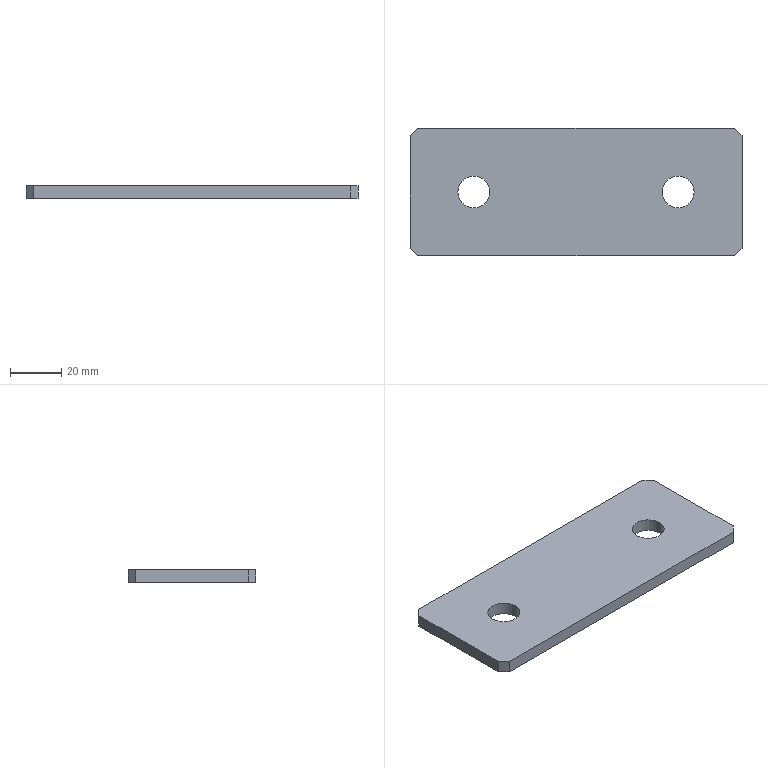Part | SolidWorks | features Extrusion 1 | 1 solid | 14 faces | box 130 x 50 x 5 mm | volume 31183 mm3 | plane 10 | cylinder 4 | commonest cylinder face diameters 12.5 x4
STEP:
#1=CARTESIAN_POINT('',(33.75,0.,-2.5));
#2=VERTEX_POINT('',#1);
#3=CARTESIAN_POINT('',(46.25,0.,-2.5));
#4=VERTEX_POINT('',#3);
#5=CARTESIAN_POINT('',(40.,0.,-2.5));
#6=DIRECTION('',(0.,0.,1.));
#7=DIRECTION('',(-1.,0.,0.));
#8=AXIS2_PLACEMENT_3D('',#5,#6,#7);
#9=CIRCLE('',#8,6.25);
#10=EDGE_CURVE('',#2,#4,#9,.T.);
#11=ORIENTED_EDGE('',*,*,#10,.F.);
#12=CARTESIAN_POINT('',(33.75,0.,2.5));
#13=VERTEX_POINT('',#12);
#14=CARTESIAN_POINT('',(33.75,0.,-2.5));
#15=DIRECTION('',(0.,0.,1.));
#16=VECTOR('',#15,1000.);
#17=LINE('',#14,#16);
#18=EDGE_CURVE('',#2,#13,#17,.T.);
#19=ORIENTED_EDGE('',*,*,#18,.T.);
#20=CARTESIAN_POINT('',(46.25,0.,2.5));
#21=VERTEX_POINT('',#20);
#22=CARTESIAN_POINT('',(40.,0.,2.5));
#23=DIRECTION('',(0.,0.,1.));
#24=DIRECTION('',(-1.,0.,0.));
#25=AXIS2_PLACEMENT_3D('',#22,#23,#24);
#26=CIRCLE('',#25,6.25);
#27=EDGE_CURVE('',#13,#21,#26,.T.);
#28=ORIENTED_EDGE('',*,*,#27,.T.);
#29=CARTESIAN_POINT('',(46.25,0.,-2.5));
#30=DIRECTION('',(0.,0.,1.));
#31=VECTOR('',#30,1000.);
#32=LINE('',#29,#31);
#33=EDGE_CURVE('',#4,#21,#32,.T.);
#34=ORIENTED_EDGE('',*,*,#33,.F.);
#35=EDGE_LOOP('',(#11,#19,#28,#34));
#36=FACE_OUTER_BOUND('',#35,.T.);
#37=CARTESIAN_POINT('',(40.,0.,-2.5));
#38=DIRECTION('',(0.,0.,1.));
#39=DIRECTION('',(1.,0.,0.));
#40=AXIS2_PLACEMENT_3D('',#37,#38,#39);
#41=CYLINDRICAL_SURFACE('',#40,6.25);
#42=ADVANCED_FACE('',(#36),#41,.F.);
#43=CARTESIAN_POINT('',(-46.25,0.,-2.5));
#44=VERTEX_POINT('',#43);
#45=CARTESIAN_POINT('',(-33.75,0.,-2.5));
#46=VERTEX_POINT('',#45);
#47=CARTESIAN_POINT('',(-40.,0.,-2.5));
#48=DIRECTION('',(0.,0.,1.));
#49=DIRECTION('',(-1.,0.,0.));
#50=AXIS2_PLACEMENT_3D('',#47,#48,#49);
#51=CIRCLE('',#50,6.25);
#52=EDGE_CURVE('',#44,#46,#51,.T.);
#53=ORIENTED_EDGE('',*,*,#52,.F.);
#54=CARTESIAN_POINT('',(-46.25,0.,2.5));
#55=VERTEX_POINT('',#54);
#56=CARTESIAN_POINT('',(-46.25,0.,-2.5));
#57=DIRECTION('',(0.,0.,1.));
#58=VECTOR('',#57,1000.);
#59=LINE('',#56,#58);
#60=EDGE_CURVE('',#44,#55,#59,.T.);
#61=ORIENTED_EDGE('',*,*,#60,.T.);
#62=CARTESIAN_POINT('',(-33.75,0.,2.5));
#63=VERTEX_POINT('',#62);
#64=CARTESIAN_POINT('',(-40.,0.,2.5));
#65=DIRECTION('',(0.,0.,1.));
#66=DIRECTION('',(-1.,0.,0.));
#67=AXIS2_PLACEMENT_3D('',#64,#65,#66);
#68=CIRCLE('',#67,6.25);
#69=EDGE_CURVE('',#55,#63,#68,.T.);
#70=ORIENTED_EDGE('',*,*,#69,.T.);
#71=CARTESIAN_POINT('',(-33.75,0.,-2.5));
#72=DIRECTION('',(0.,0.,1.));
#73=VECTOR('',#72,1000.);
#74=LINE('',#71,#73);
#75=EDGE_CURVE('',#46,#63,#74,.T.);
#76=ORIENTED_EDGE('',*,*,#75,.F.);
#77=EDGE_LOOP('',(#53,#61,#70,#76));
#78=FACE_OUTER_BOUND('',#77,.T.);
#79=CARTESIAN_POINT('',(-40.,0.,-2.5));
#80=DIRECTION('',(0.,0.,1.));
#81=DIRECTION('',(1.,0.,0.));
#82=AXIS2_PLACEMENT_3D('',#79,#80,#81);
#83=CYLINDRICAL_SURFACE('',#82,6.25);
#84=ADVANCED_FACE('',(#78),#83,.F.);
#85=CARTESIAN_POINT('',(-65.,-22.,2.5));
#86=VERTEX_POINT('',#85);
#87=CARTESIAN_POINT('',(-62.,-25.,2.5));
#88=VERTEX_POINT('',#87);
#89=CARTESIAN_POINT('',(-65.,-22.,2.5));
#90=DIRECTION('',(0.7071,-0.7071,0.));
#91=VECTOR('',#90,1000.);
#92=LINE('',#89,#91);
#93=EDGE_CURVE('',#86,#88,#92,.T.);
#94=ORIENTED_EDGE('',*,*,#93,.F.);
#95=CARTESIAN_POINT('',(-65.,-22.,-2.5));
#96=VERTEX_POINT('',#95);
#97=CARTESIAN_POINT('',(-65.,-22.,-2.5));
#98=DIRECTION('',(0.,0.,1.));
#99=VECTOR('',#98,1000.);
#100=LINE('',#97,#99);
#101=EDGE_CURVE('',#96,#86,#100,.T.);
#102=ORIENTED_EDGE('',*,*,#101,.F.);
#103=CARTESIAN_POINT('',(-62.,-25.,-2.5));
#104=VERTEX_POINT('',#103);
#105=CARTESIAN_POINT('',(-65.,-22.,-2.5));
#106=DIRECTION('',(0.7071,-0.7071,0.));
#107=VECTOR('',#106,1000.);
#108=LINE('',#105,#107);
#109=EDGE_CURVE('',#96,#104,#108,.T.);
#110=ORIENTED_EDGE('',*,*,#109,.T.);
#111=CARTESIAN_POINT('',(-62.,-25.,-2.5));
#112=DIRECTION('',(0.,0.,1.));
#113=VECTOR('',#112,1000.);
#114=LINE('',#111,#113);
#115=EDGE_CURVE('',#104,#88,#114,.T.);
#116=ORIENTED_EDGE('',*,*,#115,.T.);
#117=EDGE_LOOP('',(#94,#102,#110,#116));
#118=FACE_OUTER_BOUND('',#117,.T.);
#119=CARTESIAN_POINT('',(-65.,-22.,-2.5));
#120=DIRECTION('',(-0.7071,-0.7071,0.));
#121=DIRECTION('',(0.7071,-0.7071,0.));
#122=AXIS2_PLACEMENT_3D('',#119,#120,#121);
#123=PLANE('',#122);
#124=ADVANCED_FACE('',(#118),#123,.T.);
#125=CARTESIAN_POINT('',(-65.,22.,2.5));
#126=VERTEX_POINT('',#125);
#127=CARTESIAN_POINT('',(-65.,22.,2.5));
#128=DIRECTION('',(0.,-1.,0.));
#129=VECTOR('',#128,1000.);
#130=LINE('',#127,#129);
#131=EDGE_CURVE('',#126,#86,#130,.T.);
#132=ORIENTED_EDGE('',*,*,#131,.F.);
#133=CARTESIAN_POINT('',(-65.,22.,-2.5));
#134=VERTEX_POINT('',#133);
#135=CARTESIAN_POINT('',(-65.,22.,-2.5));
#136=DIRECTION('',(0.,0.,1.));
#137=VECTOR('',#136,1000.);
#138=LINE('',#135,#137);
#139=EDGE_CURVE('',#134,#126,#138,.T.);
#140=ORIENTED_EDGE('',*,*,#139,.F.);
#141=CARTESIAN_POINT('',(-65.,22.,-2.5));
#142=DIRECTION('',(0.,-1.,0.));
#143=VECTOR('',#142,1000.);
#144=LINE('',#141,#143);
#145=EDGE_CURVE('',#134,#96,#144,.T.);
#146=ORIENTED_EDGE('',*,*,#145,.T.);
#147=ORIENTED_EDGE('',*,*,#101,.T.);
#148=EDGE_LOOP('',(#132,#140,#146,#147));
#149=FACE_OUTER_BOUND('',#148,.T.);
#150=CARTESIAN_POINT('',(-65.,22.,-2.5));
#151=DIRECTION('',(-1.,0.,0.));
#152=DIRECTION('',(0.,0.,1.));
#153=AXIS2_PLACEMENT_3D('',#150,#151,#152);
#154=PLANE('',#153);
#155=ADVANCED_FACE('',(#149),#154,.T.);
#156=CARTESIAN_POINT('',(-62.,25.,2.5));
#157=VERTEX_POINT('',#156);
#158=CARTESIAN_POINT('',(-62.,25.,2.5));
#159=DIRECTION('',(-0.7071,-0.7071,0.));
#160=VECTOR('',#159,1000.);
#161=LINE('',#158,#160);
#162=EDGE_CURVE('',#157,#126,#161,.T.);
#163=ORIENTED_EDGE('',*,*,#162,.F.);
#164=CARTESIAN_POINT('',(-62.,25.,-2.5));
#165=VERTEX_POINT('',#164);
#166=CARTESIAN_POINT('',(-62.,25.,-2.5));
#167=DIRECTION('',(0.,0.,1.));
#168=VECTOR('',#167,1000.);
#169=LINE('',#166,#168);
#170=EDGE_CURVE('',#165,#157,#169,.T.);
#171=ORIENTED_EDGE('',*,*,#170,.F.);
#172=CARTESIAN_POINT('',(-62.,25.,-2.5));
#173=DIRECTION('',(-0.7071,-0.7071,0.));
#174=VECTOR('',#173,1000.);
#175=LINE('',#172,#174);
#176=EDGE_CURVE('',#165,#134,#175,.T.);
#177=ORIENTED_EDGE('',*,*,#176,.T.);
#178=ORIENTED_EDGE('',*,*,#139,.T.);
#179=EDGE_LOOP('',(#163,#171,#177,#178));
#180=FACE_OUTER_BOUND('',#179,.T.);
#181=CARTESIAN_POINT('',(-62.,25.,-2.5));
#182=DIRECTION('',(-0.7071,0.7071,0.));
#183=DIRECTION('',(-0.7071,-0.7071,0.));
#184=AXIS2_PLACEMENT_3D('',#181,#182,#183);
#185=PLANE('',#184);
#186=ADVANCED_FACE('',(#180),#185,.T.);
#187=CARTESIAN_POINT('',(62.,25.,2.5));
#188=VERTEX_POINT('',#187);
#189=CARTESIAN_POINT('',(62.,25.,2.5));
#190=DIRECTION('',(-1.,0.,0.));
#191=VECTOR('',#190,1000.);
#192=LINE('',#189,#191);
#193=EDGE_CURVE('',#188,#157,#192,.T.);
#194=ORIENTED_EDGE('',*,*,#193,.F.);
#195=CARTESIAN_POINT('',(62.,25.,-2.5));
#196=VERTEX_POINT('',#195);
#197=CARTESIAN_POINT('',(62.,25.,-2.5));
#198=DIRECTION('',(0.,0.,1.));
#199=VECTOR('',#198,1000.);
#200=LINE('',#197,#199);
#201=EDGE_CURVE('',#196,#188,#200,.T.);
#202=ORIENTED_EDGE('',*,*,#201,.F.);
#203=CARTESIAN_POINT('',(62.,25.,-2.5));
#204=DIRECTION('',(-1.,0.,0.));
#205=VECTOR('',#204,1000.);
#206=LINE('',#203,#205);
#207=EDGE_CURVE('',#196,#165,#206,.T.);
#208=ORIENTED_EDGE('',*,*,#207,.T.);
#209=ORIENTED_EDGE('',*,*,#170,.T.);
#210=EDGE_LOOP('',(#194,#202,#208,#209));
#211=FACE_OUTER_BOUND('',#210,.T.);
#212=CARTESIAN_POINT('',(62.,25.,-2.5));
#213=DIRECTION('',(0.,1.,0.));
#214=DIRECTION('',(0.,0.,1.));
#215=AXIS2_PLACEMENT_3D('',#212,#213,#214);
#216=PLANE('',#215);
#217=ADVANCED_FACE('',(#211),#216,.T.);
#218=CARTESIAN_POINT('',(65.,22.,2.5));
#219=VERTEX_POINT('',#218);
#220=CARTESIAN_POINT('',(65.,22.,2.5));
#221=DIRECTION('',(-0.7071,0.7071,0.));
#222=VECTOR('',#221,1000.);
#223=LINE('',#220,#222);
#224=EDGE_CURVE('',#219,#188,#223,.T.);
#225=ORIENTED_EDGE('',*,*,#224,.F.);
#226=CARTESIAN_POINT('',(65.,22.,-2.5));
#227=VERTEX_POINT('',#226);
#228=CARTESIAN_POINT('',(65.,22.,-2.5));
#229=DIRECTION('',(0.,0.,1.));
#230=VECTOR('',#229,1000.);
#231=LINE('',#228,#230);
#232=EDGE_CURVE('',#227,#219,#231,.T.);
#233=ORIENTED_EDGE('',*,*,#232,.F.);
#234=CARTESIAN_POINT('',(65.,22.,-2.5));
#235=DIRECTION('',(-0.7071,0.7071,0.));
#236=VECTOR('',#235,1000.);
#237=LINE('',#234,#236);
#238=EDGE_CURVE('',#227,#196,#237,.T.);
#239=ORIENTED_EDGE('',*,*,#238,.T.);
#240=ORIENTED_EDGE('',*,*,#201,.T.);
#241=EDGE_LOOP('',(#225,#233,#239,#240));
#242=FACE_OUTER_BOUND('',#241,.T.);
#243=CARTESIAN_POINT('',(65.,22.,-2.5));
#244=DIRECTION('',(0.7071,0.7071,0.));
#245=DIRECTION('',(-0.7071,0.7071,0.));
#246=AXIS2_PLACEMENT_3D('',#243,#244,#245);
#247=PLANE('',#246);
#248=ADVANCED_FACE('',(#242),#247,.T.);
#249=CARTESIAN_POINT('',(65.,-22.,2.5));
#250=VERTEX_POINT('',#249);
#251=CARTESIAN_POINT('',(65.,-22.,2.5));
#252=DIRECTION('',(0.,1.,0.));
#253=VECTOR('',#252,1000.);
#254=LINE('',#251,#253);
#255=EDGE_CURVE('',#250,#219,#254,.T.);
#256=ORIENTED_EDGE('',*,*,#255,.F.);
#257=CARTESIAN_POINT('',(65.,-22.,-2.5));
#258=VERTEX_POINT('',#257);
#259=CARTESIAN_POINT('',(65.,-22.,-2.5));
#260=DIRECTION('',(0.,0.,1.));
#261=VECTOR('',#260,1000.);
#262=LINE('',#259,#261);
#263=EDGE_CURVE('',#258,#250,#262,.T.);
#264=ORIENTED_EDGE('',*,*,#263,.F.);
#265=CARTESIAN_POINT('',(65.,-22.,-2.5));
#266=DIRECTION('',(0.,1.,0.));
#267=VECTOR('',#266,1000.);
#268=LINE('',#265,#267);
#269=EDGE_CURVE('',#258,#227,#268,.T.);
#270=ORIENTED_EDGE('',*,*,#269,.T.);
#271=ORIENTED_EDGE('',*,*,#232,.T.);
#272=EDGE_LOOP('',(#256,#264,#270,#271));
#273=FACE_OUTER_BOUND('',#272,.T.);
#274=CARTESIAN_POINT('',(65.,-22.,-2.5));
#275=DIRECTION('',(1.,0.,0.));
#276=DIRECTION('',(0.,0.,-1.));
#277=AXIS2_PLACEMENT_3D('',#274,#275,#276);
#278=PLANE('',#277);
#279=ADVANCED_FACE('',(#273),#278,.T.);
#280=CARTESIAN_POINT('',(62.,-25.,2.5));
#281=VERTEX_POINT('',#280);
#282=CARTESIAN_POINT('',(62.,-25.,2.5));
#283=DIRECTION('',(0.7071,0.7071,0.));
#284=VECTOR('',#283,1000.);
#285=LINE('',#282,#284);
#286=EDGE_CURVE('',#281,#250,#285,.T.);
#287=ORIENTED_EDGE('',*,*,#286,.F.);
#288=CARTESIAN_POINT('',(62.,-25.,-2.5));
#289=VERTEX_POINT('',#288);
#290=CARTESIAN_POINT('',(62.,-25.,-2.5));
#291=DIRECTION('',(0.,0.,1.));
#292=VECTOR('',#291,1000.);
#293=LINE('',#290,#292);
#294=EDGE_CURVE('',#289,#281,#293,.T.);
#295=ORIENTED_EDGE('',*,*,#294,.F.);
#296=CARTESIAN_POINT('',(62.,-25.,-2.5));
#297=DIRECTION('',(0.7071,0.7071,0.));
#298=VECTOR('',#297,1000.);
#299=LINE('',#296,#298);
#300=EDGE_CURVE('',#289,#258,#299,.T.);
#301=ORIENTED_EDGE('',*,*,#300,.T.);
#302=ORIENTED_EDGE('',*,*,#263,.T.);
#303=EDGE_LOOP('',(#287,#295,#301,#302));
#304=FACE_OUTER_BOUND('',#303,.T.);
#305=CARTESIAN_POINT('',(62.,-25.,-2.5));
#306=DIRECTION('',(0.7071,-0.7071,0.));
#307=DIRECTION('',(0.7071,0.7071,0.));
#308=AXIS2_PLACEMENT_3D('',#305,#306,#307);
#309=PLANE('',#308);
#310=ADVANCED_FACE('',(#304),#309,.T.);
#311=CARTESIAN_POINT('',(-62.,-25.,2.5));
#312=DIRECTION('',(1.,0.,0.));
#313=VECTOR('',#312,1000.);
#314=LINE('',#311,#313);
#315=EDGE_CURVE('',#88,#281,#314,.T.);
#316=ORIENTED_EDGE('',*,*,#315,.F.);
#317=ORIENTED_EDGE('',*,*,#115,.F.);
#318=CARTESIAN_POINT('',(-62.,-25.,-2.5));
#319=DIRECTION('',(1.,0.,0.));
#320=VECTOR('',#319,1000.);
#321=LINE('',#318,#320);
#322=EDGE_CURVE('',#104,#289,#321,.T.);
#323=ORIENTED_EDGE('',*,*,#322,.T.);
#324=ORIENTED_EDGE('',*,*,#294,.T.);
#325=EDGE_LOOP('',(#316,#317,#323,#324));
#326=FACE_OUTER_BOUND('',#325,.T.);
#327=CARTESIAN_POINT('',(-62.,-25.,-2.5));
#328=DIRECTION('',(0.,-1.,0.));
#329=DIRECTION('',(0.,0.,-1.));
#330=AXIS2_PLACEMENT_3D('',#327,#328,#329);
#331=PLANE('',#330);
#332=ADVANCED_FACE('',(#326),#331,.T.);
#333=CARTESIAN_POINT('',(40.,0.,-2.5));
#334=DIRECTION('',(0.,0.,1.));
#335=DIRECTION('',(-1.,0.,0.));
#336=AXIS2_PLACEMENT_3D('',#333,#334,#335);
#337=CIRCLE('',#336,6.25);
#338=EDGE_CURVE('',#4,#2,#337,.T.);
#339=ORIENTED_EDGE('',*,*,#338,.T.);
#340=ORIENTED_EDGE('',*,*,#10,.T.);
#341=EDGE_LOOP('',(#339,#340));
#342=FACE_BOUND('',#341,.T.);
#343=CARTESIAN_POINT('',(-40.,0.,-2.5));
#344=DIRECTION('',(0.,0.,1.));
#345=DIRECTION('',(-1.,0.,0.));
#346=AXIS2_PLACEMENT_3D('',#343,#344,#345);
#347=CIRCLE('',#346,6.25);
#348=EDGE_CURVE('',#46,#44,#347,.T.);
#349=ORIENTED_EDGE('',*,*,#348,.T.);
#350=ORIENTED_EDGE('',*,*,#52,.T.);
#351=EDGE_LOOP('',(#349,#350));
#352=FACE_BOUND('',#351,.T.);
#353=ORIENTED_EDGE('',*,*,#109,.F.);
#354=ORIENTED_EDGE('',*,*,#145,.F.);
#355=ORIENTED_EDGE('',*,*,#176,.F.);
#356=ORIENTED_EDGE('',*,*,#207,.F.);
#357=ORIENTED_EDGE('',*,*,#238,.F.);
#358=ORIENTED_EDGE('',*,*,#269,.F.);
#359=ORIENTED_EDGE('',*,*,#300,.F.);
#360=ORIENTED_EDGE('',*,*,#322,.F.);
#361=EDGE_LOOP('',(#353,#354,#355,#356,#357,#358,#359,#360));
#362=FACE_OUTER_BOUND('',#361,.T.);
#363=CARTESIAN_POINT('',(0.,0.,-2.5));
#364=DIRECTION('',(0.,0.,1.));
#365=DIRECTION('',(1.,0.,0.));
#366=AXIS2_PLACEMENT_3D('',#363,#364,#365);
#367=PLANE('',#366);
#368=ADVANCED_FACE('',(#342,#352,#362),#367,.F.);
#369=CARTESIAN_POINT('',(40.,0.,2.5));
#370=DIRECTION('',(0.,0.,1.));
#371=DIRECTION('',(-1.,0.,0.));
#372=AXIS2_PLACEMENT_3D('',#369,#370,#371);
#373=CIRCLE('',#372,6.25);
#374=EDGE_CURVE('',#21,#13,#373,.T.);
#375=ORIENTED_EDGE('',*,*,#374,.F.);
#376=ORIENTED_EDGE('',*,*,#27,.F.);
#377=EDGE_LOOP('',(#375,#376));
#378=FACE_BOUND('',#377,.T.);
#379=CARTESIAN_POINT('',(-40.,0.,2.5));
#380=DIRECTION('',(0.,0.,1.));
#381=DIRECTION('',(-1.,0.,0.));
#382=AXIS2_PLACEMENT_3D('',#379,#380,#381);
#383=CIRCLE('',#382,6.25);
#384=EDGE_CURVE('',#63,#55,#383,.T.);
#385=ORIENTED_EDGE('',*,*,#384,.F.);
#386=ORIENTED_EDGE('',*,*,#69,.F.);
#387=EDGE_LOOP('',(#385,#386));
#388=FACE_BOUND('',#387,.T.);
#389=ORIENTED_EDGE('',*,*,#93,.T.);
#390=ORIENTED_EDGE('',*,*,#315,.T.);
#391=ORIENTED_EDGE('',*,*,#286,.T.);
#392=ORIENTED_EDGE('',*,*,#255,.T.);
#393=ORIENTED_EDGE('',*,*,#224,.T.);
#394=ORIENTED_EDGE('',*,*,#193,.T.);
#395=ORIENTED_EDGE('',*,*,#162,.T.);
#396=ORIENTED_EDGE('',*,*,#131,.T.);
#397=EDGE_LOOP('',(#389,#390,#391,#392,#393,#394,#395,#396));
#398=FACE_OUTER_BOUND('',#397,.T.);
#399=CARTESIAN_POINT('',(0.,0.,2.5));
#400=DIRECTION('',(0.,0.,1.));
#401=DIRECTION('',(1.,0.,0.));
#402=AXIS2_PLACEMENT_3D('',#399,#400,#401);
#403=PLANE('',#402);
#404=ADVANCED_FACE('',(#378,#388,#398),#403,.T.);
#405=ORIENTED_EDGE('',*,*,#60,.F.);
#406=ORIENTED_EDGE('',*,*,#348,.F.);
#407=ORIENTED_EDGE('',*,*,#75,.T.);
#408=ORIENTED_EDGE('',*,*,#384,.T.);
#409=EDGE_LOOP('',(#405,#406,#407,#408));
#410=FACE_OUTER_BOUND('',#409,.T.);
#411=CARTESIAN_POINT('',(-40.,0.,-2.5));
#412=DIRECTION('',(0.,0.,1.));
#413=DIRECTION('',(1.,0.,0.));
#414=AXIS2_PLACEMENT_3D('',#411,#412,#413);
#415=CYLINDRICAL_SURFACE('',#414,6.25);
#416=ADVANCED_FACE('',(#410),#415,.F.);
#417=ORIENTED_EDGE('',*,*,#18,.F.);
#418=ORIENTED_EDGE('',*,*,#338,.F.);
#419=ORIENTED_EDGE('',*,*,#33,.T.);
#420=ORIENTED_EDGE('',*,*,#374,.T.);
#421=EDGE_LOOP('',(#417,#418,#419,#420));
#422=FACE_OUTER_BOUND('',#421,.T.);
#423=CARTESIAN_POINT('',(40.,0.,-2.5));
#424=DIRECTION('',(0.,0.,1.));
#425=DIRECTION('',(1.,0.,0.));
#426=AXIS2_PLACEMENT_3D('',#423,#424,#425);
#427=CYLINDRICAL_SURFACE('',#426,6.25);
#428=ADVANCED_FACE('',(#422),#427,.F.);
#429=CLOSED_SHELL('',(#42,#84,#124,#155,#186,#217,#248,#279,#310,#332,#368,#404,#416,#428));
#430=MANIFOLD_SOLID_BREP('',#429);
#431=CARTESIAN_POINT('',(0.,0.,0.));
#432=DIRECTION('',(0.,0.,1.));
#433=DIRECTION('',(1.,0.,0.));
#434=AXIS2_PLACEMENT_3D('',#431,#432,#433);
#435=(LENGTH_UNIT()NAMED_UNIT(*)SI_UNIT(.MILLI.,.METRE.));
#436=UNCERTAINTY_MEASURE_WITH_UNIT(LENGTH_MEASURE(0.00001),#435,'','');
#437=(NAMED_UNIT(*)PLANE_ANGLE_UNIT()SI_UNIT($,.RADIAN.));
#438=(NAMED_UNIT(*)SI_UNIT($,.STERADIAN.)SOLID_ANGLE_UNIT());
#439=(GEOMETRIC_REPRESENTATION_CONTEXT(3)GLOBAL_UNCERTAINTY_ASSIGNED_CONTEXT((#436))GLOBAL_UNIT_ASSIGNED_CONTEXT((#435,#437,#438))REPRESENTATION_CONTEXT('',''));
#440=ADVANCED_BREP_SHAPE_REPRESENTATION('',(#430,#434),#439);